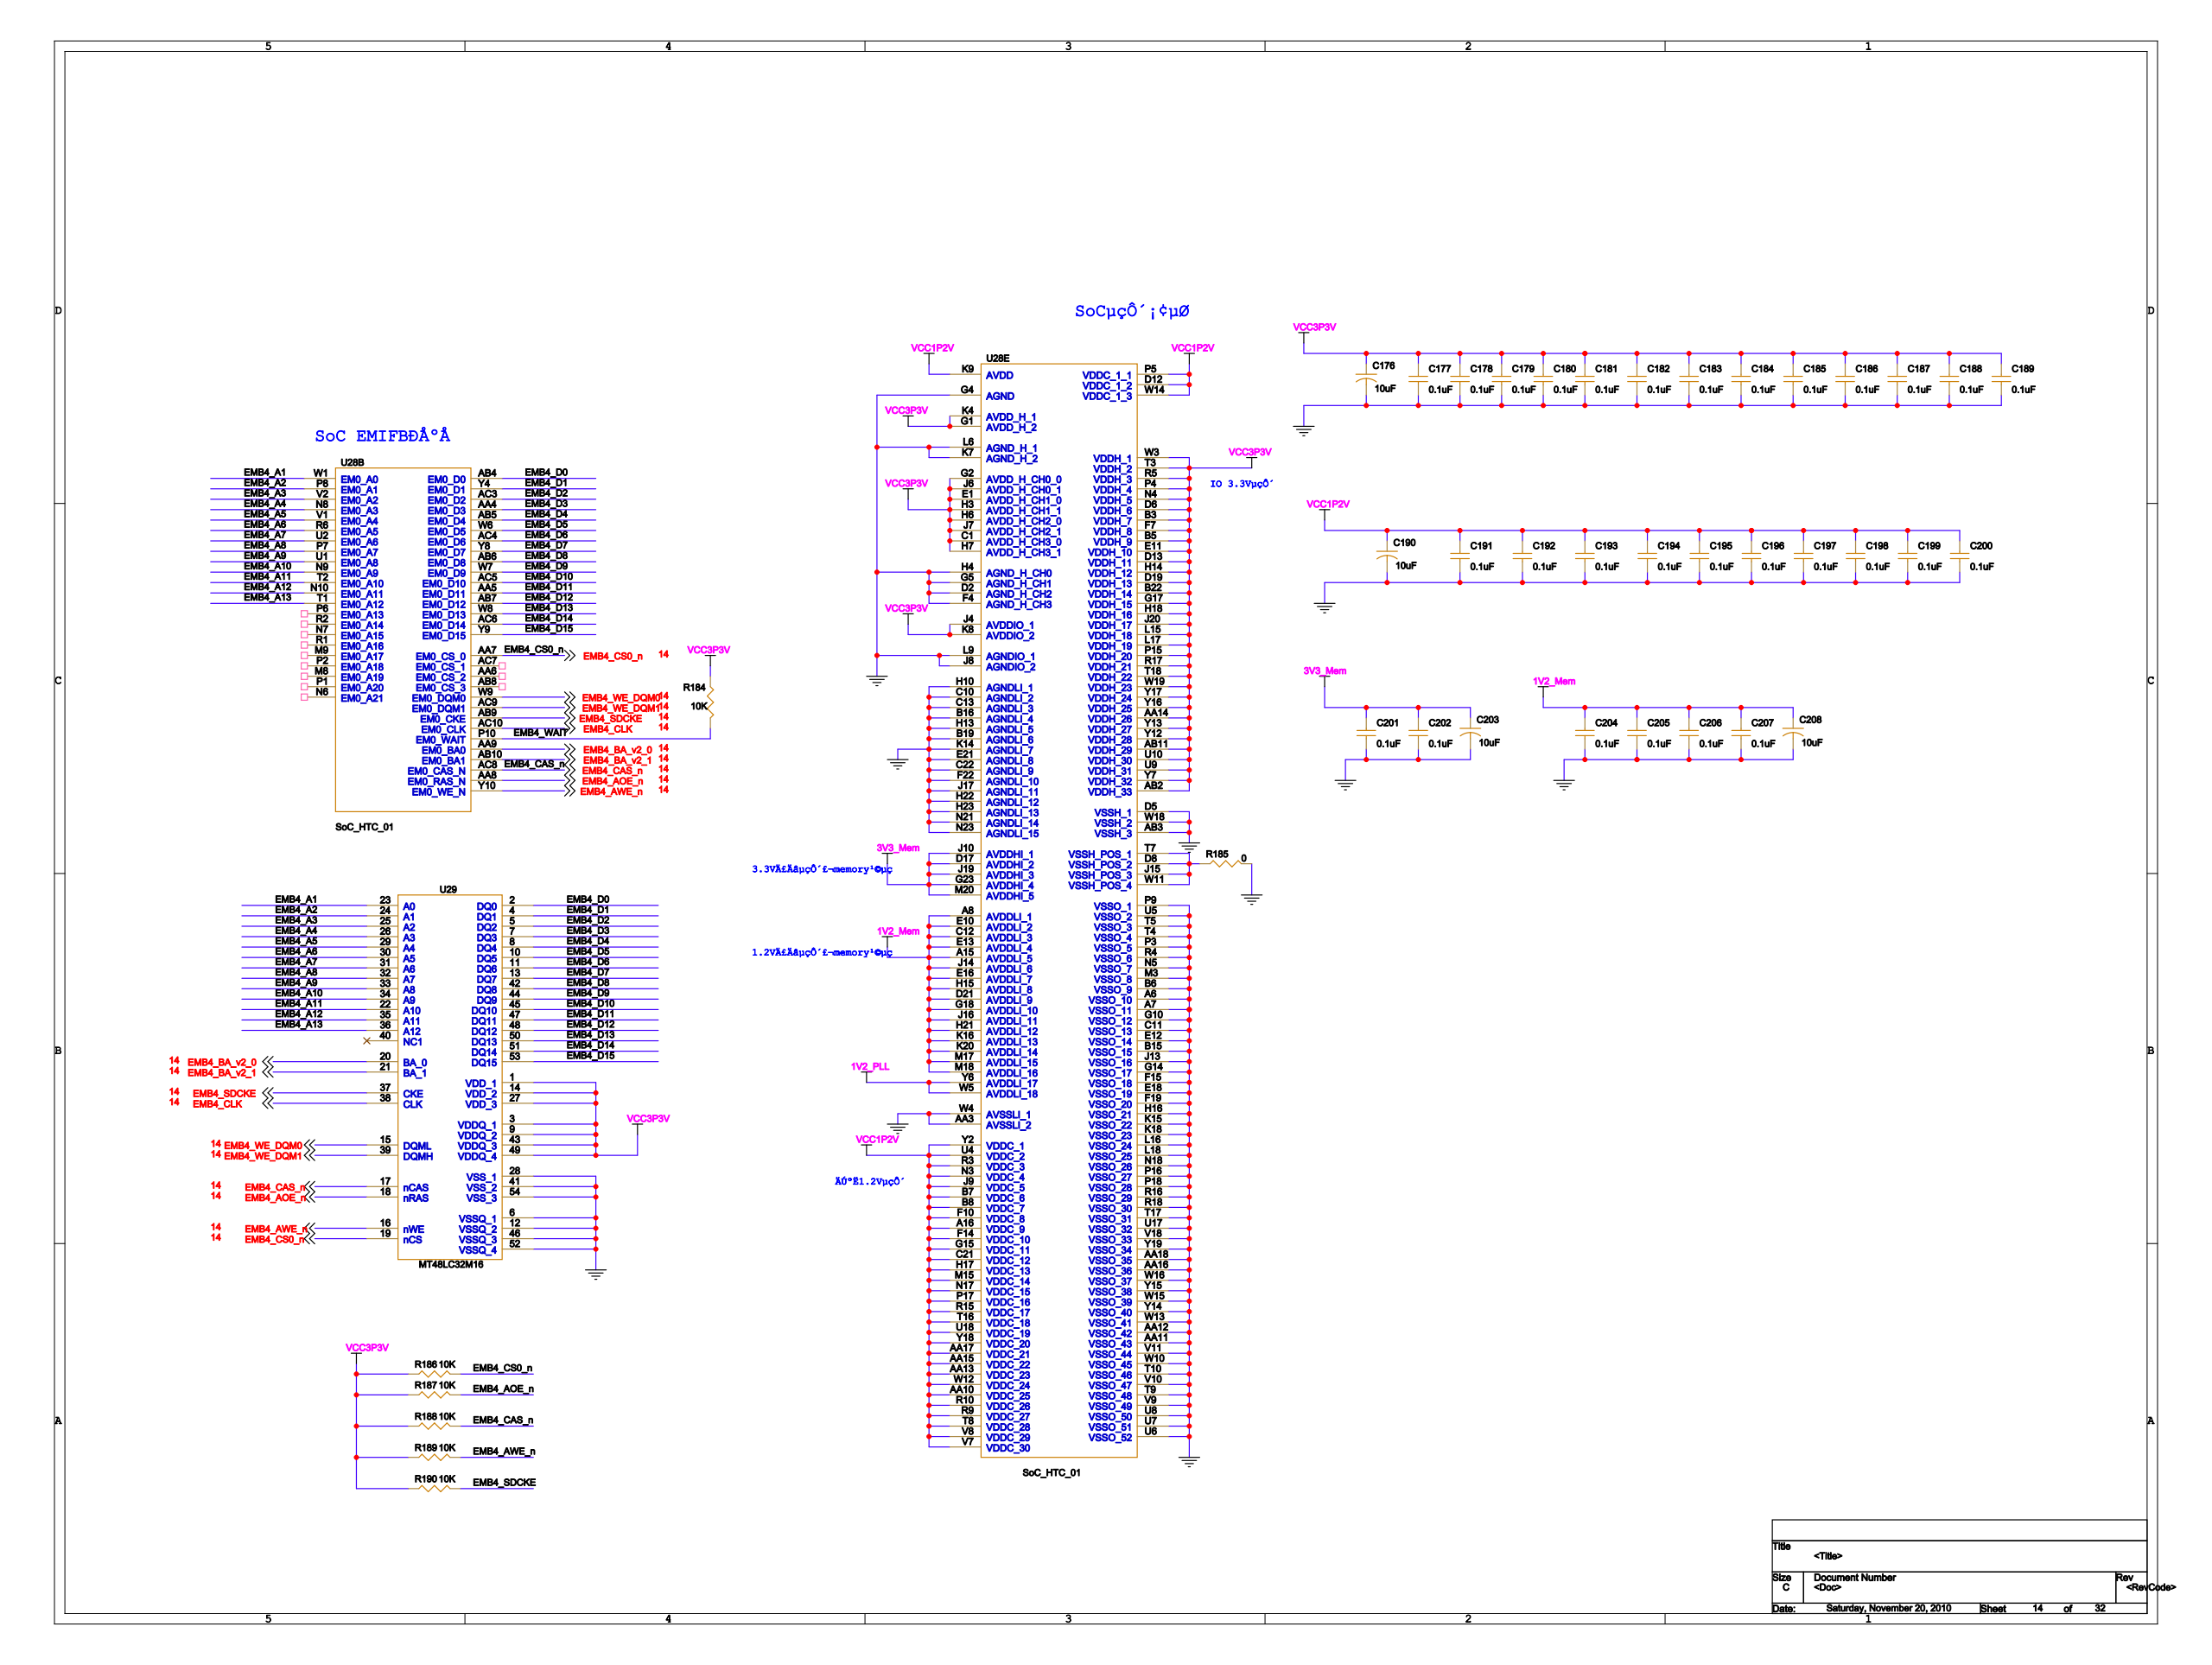Circuit board | Cadence Allegro | 1001 parts | 1318 nets | one sheet of the schematic
Parts on this sheet (reference | value | footprint):
C176 | 10uF | C3216
C177 | 0.1uF | C0402
C178 | 0.1uF | C0402
C179 | 0.1uF | C0402
C180 | 0.1uF | C0402
C181 | 0.1uF | C0402
C182 | 0.1uF | C0402
C183 | 0.1uF | C0402
C184 | 0.1uF | C0402
C185 | 0.1uF | C0402
C186 | 0.1uF | C0402
C187 | 0.1uF | C0402
C188 | 0.1uF | C0402
C189 | 0.1uF | C0402
C190 | 10uF | C3216
C191 | 0.1uF | C0402
C192 | 0.1uF | C0402
C193 | 0.1uF | C0402
C194 | 0.1uF | C0402
C195 | 0.1uF | C0402
C196 | 0.1uF | C0402
C197 | 0.1uF | C0402
C198 | 0.1uF | C0402
C199 | 0.1uF | C0402
C200 | 0.1uF | C0402
C201 | 0.1uF | C0402
C202 | 0.1uF | C0402
C203 | 10uF | C3216
C204 | 0.1uF | C0402
C205 | 0.1uF | C0402
C206 | 0.1uF | C0402
C207 | 0.1uF | C0402
C208 | 10uF | C3216
R184 | 10K | 0603
R185 | 0 | 0603
R186 | 10K | 0603
R187 | 10K | 0603
R188 | 10K | 0603
R189 | 10K | 0603
R190 | 10K | 0603
U1 | SoC_HTC_01 | L529_XIN
U2 | MT48LC32M16 | TSOP54
U4 | MAX3243 | TSSOP-28
U6 | MT48LC16M16 | TSOP54
U7 | MT48LC16M16 | TSOP54
U8 | DP83848C | DP83848C_48LQFP
U10 | SoC_HTC_01 | L529_XIN
U17 | MT48LC32M16 | TSOP54
U28 | SoC_HTC_01 | L529_XIN
U29 | MT48LC32M16 | TSOP54
Nets of these parts (net: part-pin ...):
GND: C176-2 C177-2 C178-2 C179-2 C180-2 C181-2 C182-2 C183-2 C184-2 C185-2 C186-2 C187-2 C188-2 C189-2 C190-2 C191-2 C192-2 C193-2 C194-2 C195-2 C196-2 C197-2 C198-2 C199-2 C200-2 C201-2 C202-2 C203-2 C204-2 C205-2 C206-2 C207-2 C208-2 R185-2 U1-A6 U1-A7 U1-AA3 U1-AA11 U1-AA12 U1-AA16 U1-AA18 U1-AB3 U1-B6 U1-B15 U1-B16 U1-B19 U1-C10 U1-C11 U1-C13 U1-C22 U1-D2 U1-D5 U1-E12 U1-E18 U1-E21 U1-F4 U1-F15 U1-F19 U1-F22 U1-G4 U1-G5 U1-G10 U1-G14 U1-H4 U1-H10 U1-H13 U1-H16 U1-H22 U1-H23 U1-J8 U1-J13 U1-J17 U1-K7 U1-K14 U1-K15 U1-K18 U1-L6 U1-L9 U1-L16 U1-L18 U1-M3 U1-N5 U1-N18 U1-N21 U1-N23 U1-P3 U1-P9 U1-P16 U1-P18 U1-R4 U1-R16 U1-R18 U1-T4 U1-T5 U1-T9 U1-T10 U1-T17 U1-U5 U1-U6 U1-U7 U1-U8 U1-U17 U1-V9 U1-V10 U1-V11 U1-V18 U1-W4 U1-W10 U1-W13 U1-W15 U1-W16 U1-W18 U1-Y14 U1-Y15 U1-Y19 U2-6 U2-12 U2-28 U2-41 U2-46 U2-52 U2-54 U4-23 U4-25 U6-6 U6-12 U6-28 U6-41 U6-46 U6-52 U6-54 U7-6 U7-12 U7-28 U7-41 U7-46 U7-52 U7-54 U8-15 U8-19 U8-35 U8-36 U8-47 U10-A6 U10-A7 U10-AA3 U10-AA11 U10-AA12 U10-AA16 U10-AA18 U10-AB3 U10-B6 U10-B15 U10-B16 U10-B19 U10-C10 U10-C11 U10-C13 U10-C22 U10-D2 U10-D5 U10-E12 U10-E18 U10-E21 U10-F4 U10-F15 U10-F19 U10-F22 U10-G4 U10-G5 U10-G10 U10-G14 U10-H4 U10-H10 U10-H13 U10-H16 U10-H22 U10-H23 U10-J8 U10-J13 U10-J17 U10-K7 U10-K14 U10-K15 U10-K18 U10-L6 U10-L9 U10-L16 U10-L18 U10-M3 U10-N5 U10-N18 U10-N21 U10-N23 U10-P3 U10-P9 U10-P16 U10-P18 U10-R4 U10-R16 U10-R18 U10-T4 U10-T5 U10-T9 U10-T10 U10-T17 U10-U5 U10-U6 U10-U7 U10-U8 U10-U17 U10-V9 U10-V10 U10-V11 U10-V18 U10-W4 U10-W10 U10-W13 U10-W15 U10-W16 U10-W18 U10-Y14 U10-Y15 U10-Y19 U17-6 U17-12 U17-28 U17-41 U17-46 U17-52 U17-54 U28-A6 U28-A7 U28-AA3 U28-AA11 U28-AA12 U28-AA16 U28-AA18 U28-AB3 U28-B6 U28-B15 U28-B16 U28-B19 U28-C10 U28-C11 U28-C13 U28-C22 U28-D2 U28-D5 U28-E12 U28-E18 U28-E21 U28-F4 U28-F15 U28-F19 U28-F22 U28-G4 U28-G5 U28-G10 U28-G14 U28-H4 U28-H10 U28-H13 U28-H16 U28-H22 U28-H23 U28-J8 U28-J13 U28-J17 U28-K7 U28-K14 U28-K15 U28-K18 U28-L6 U28-L9 U28-L16 U28-L18 U28-M3 U28-N5 U28-N18 U28-N21 U28-N23 U28-P3 U28-P9 U28-P16 U28-P18 U28-R4 U28-R16 U28-R18 U28-T4 U28-T5 U28-T9 U28-T10 U28-T17 U28-U5 U28-U6 U28-U7 U28-U8 U28-U17 U28-V9 U28-V10 U28-V11 U28-V18 U28-W4 U28-W10 U28-W13 U28-W15 U28-W16 U28-W18 U28-Y14 U28-Y15 U28-Y19 U29-6 U29-12 U29-28 U29-41 U29-46 U29-52 U29-54
VCC3P3V: C176-1 C177-1 C178-1 C179-1 C180-1 C181-1 C182-1 C183-1 C184-1 C185-1 C186-1 C187-1 C188-1 C189-1 R184-2 R186-1 R187-1 R188-1 R189-1 R190-1 U1-AA14 U1-AB2 U1-AB11 U1-B3 U1-B5 U1-B22 U1-C1 U1-D6 U1-D13 U1-D19 U1-E1 U1-E11 U1-F7 U1-G1 U1-G2 U1-G17 U1-H3 U1-H6 U1-H7 U1-H14 U1-H18 U1-J4 U1-J6 U1-J7 U1-J20 U1-K4 U1-K8 U1-L15 U1-L17 U1-N4 U1-P4 U1-P15 U1-R5 U1-R17 U1-T3 U1-T18 U1-U9 U1-U10 U1-W3 U1-W19 U1-Y7 U1-Y12 U1-Y13 U1-Y16 U1-Y17 U2-1 U2-3 U2-9 U2-14 U2-27 U2-43 U2-49 U4-22 U4-26 U6-1 U6-3 U6-9 U6-14 U6-27 U6-43 U6-49 U7-1 U7-3 U7-9 U7-14 U7-27 U7-43 U7-49 U8-22 U8-32 U8-48 U10-AA14 U10-AB2 U10-AB11 U10-B3 U10-B5 U10-B22 U10-C1 U10-D6 U10-D13 U10-D19 U10-E1 U10-E11 U10-F7 U10-G1 U10-G2 U10-G17 U10-H3 U10-H6 U10-H7 U10-H14 U10-H18 U10-J4 U10-J6 U10-J7 U10-J20 U10-K4 U10-K8 U10-L15 U10-L17 U10-N4 U10-P4 U10-P15 U10-R5 U10-R17 U10-T3 U10-T18 U10-U9 U10-U10 U10-W3 U10-W19 U10-Y7 U10-Y12 U10-Y13 U10-Y16 U10-Y17 U17-1 U17-3 U17-9 U17-14 U17-27 U17-43 U17-49 U28-AA14 U28-AB2 U28-AB11 U28-B3 U28-B5 U28-B22 U28-C1 U28-D6 U28-D13 U28-D19 U28-E1 U28-E11 U28-F7 U28-G1 U28-G2 U28-G17 U28-H3 U28-H6 U28-H7 U28-H14 U28-H18 U28-J4 U28-J6 U28-J7 U28-J20 U28-K4 U28-K8 U28-L15 U28-L17 U28-N4 U28-P4 U28-P15 U28-R5 U28-R17 U28-T3 U28-T18 U28-U9 U28-U10 U28-W3 U28-W19 U28-Y7 U28-Y12 U28-Y13 U28-Y16 U28-Y17 U29-1 U29-3 U29-9 U29-14 U29-27 U29-43 U29-49
VCC1P2V: C190-1 C191-1 C192-1 C193-1 C194-1 C195-1 C196-1 C197-1 C198-1 C199-1 C200-1 U1-A16 U1-AA10 U1-AA13 U1-AA15 U1-AA17 U1-B7 U1-B8 U1-C21 U1-D12 U1-F10 U1-F14 U1-G15 U1-H17 U1-J9 U1-K9 U1-M15 U1-N3 U1-N17 U1-P5 U1-P17 U1-R3 U1-R9 U1-R10 U1-R15 U1-T8 U1-T16 U1-U4 U1-U18 U1-V7 U1-V8 U1-W12 U1-W14 U1-Y2 U1-Y18 U10-A16 U10-AA10 U10-AA13 U10-AA15 U10-AA17 U10-B7 U10-B8 U10-C21 U10-D12 U10-F10 U10-F14 U10-G15 U10-H17 U10-J9 U10-K9 U10-M15 U10-N3 U10-N17 U10-P5 U10-P17 U10-R3 U10-R9 U10-R10 U10-R15 U10-T8 U10-T16 U10-U4 U10-U18 U10-V7 U10-V8 U10-W12 U10-W14 U10-Y2 U10-Y18 U28-A16 U28-AA10 U28-AA13 U28-AA15 U28-AA17 U28-B7 U28-B8 U28-C21 U28-D12 U28-F10 U28-F14 U28-G15 U28-H17 U28-J9 U28-K9 U28-M15 U28-N3 U28-N17 U28-P5 U28-P17 U28-R3 U28-R9 U28-R10 U28-R15 U28-T8 U28-T16 U28-U4 U28-U18 U28-V7 U28-V8 U28-W12 U28-W14 U28-Y2 U28-Y18
3V3_MEM: C201-1 C202-1 C203-1 U1-D17 U1-G23 U1-J10 U1-J19 U1-M20 U10-D17 U10-G23 U10-J10 U10-J19 U10-M20 U28-D17 U28-G23 U28-J10 U28-J19 U28-M20
1V2_MEM: C204-1 C205-1 C206-1 C207-1 C208-1 U1-A8 U1-A15 U1-C12 U1-D21 U1-E10 U1-E13 U1-E16 U1-G18 U1-H15 U1-H21 U1-J14 U1-J16 U1-K16 U1-K20 U1-M17 U1-M18 U10-A8 U10-A15 U10-C12 U10-D21 U10-E10 U10-E13 U10-E16 U10-G18 U10-H15 U10-H21 U10-J14 U10-J16 U10-K16 U10-K20 U10-M17 U10-M18 U28-A8 U28-A15 U28-C12 U28-D21 U28-E10 U28-E13 U28-E16 U28-G18 U28-H15 U28-H21 U28-J14 U28-J16 U28-K16 U28-K20 U28-M17 U28-M18
1V2_PLL: U1-W5 U1-Y6 U10-W5 U10-Y6 U28-W5 U28-Y6
EMB4_A1: U28-W1 U29-23
EMB4_A2: U28-P8 U29-24
EMB4_A11: U28-T2 U29-22
EMB4_A12: U28-N10 U29-35
EMB4_A13: U28-T1 U29-36
EMB4_A3: U28-V2 U29-25
EMB4_A4: U28-N8 U29-26
EMB4_A5: U28-V1 U29-29
EMB4_A6: U28-R6 U29-30
EMB4_A7: U28-U2 U29-31
EMB4_A8: U28-P7 U29-32
EMB4_A9: U28-U1 U29-33
EMB4_A10: U28-N9 U29-34
EMB4_CAS_N: R188-2 U28-AC8 U29-17
EMB4_SDCKE: R190-2 U28-AB9 U29-37
EMB4_CLK: U28-AC10 U29-38
EMB4_CS0_N: R186-2 U28-AA7 U29-19
EMB4_D0: U28-AB4 U29-2
EMB4_D1: U28-Y4 U29-4
EMB4_D10: U28-AC5 U29-45
EMB4_D11: U28-AA5 U29-47
EMB4_D12: U28-AB7 U29-48
EMB4_D13: U28-W8 U29-50
EMB4_D14: U28-AC6 U29-51
EMB4_D15: U28-Y9 U29-53
EMB4_D2: U28-AC3 U29-5
EMB4_D3: U28-AA4 U29-7
EMB4_D4: U28-AB5 U29-8
EMB4_D5: U28-W6 U29-10
EMB4_D6: U28-AC4 U29-11
EMB4_D7: U28-Y8 U29-13
EMB4_D8: U28-AB6 U29-42
EMB4_D9: U28-W7 U29-44
EMB4_WE_DQM0: U28-W9 U29-15
EMB4_WE_DQM1: U28-AC9 U29-39
EMB4_AOE_N: R187-2 U28-AA8 U29-18
EMB4_WAIT: R184-1 U28-P10
EMB4_AWE_N: R189-2 U28-Y10 U29-16
N17407639: R185-1 U28-D8 U28-J15 U28-T7 U28-W11